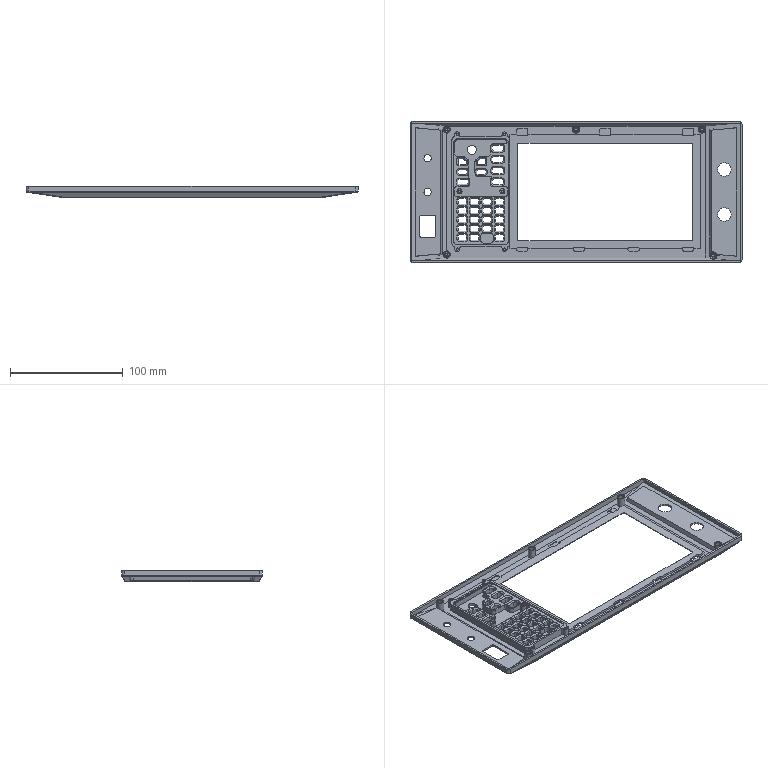NC program | NX | posted with a generic post | part box 295 x 125 x 10 mm
Lines 75 to 1153 of 134431:
(ADAPTIVE_MILLING , TOOL : D10)
N130 T10 M6
N132 G54
N134 G17 G0 G90 X-158.197 Y-0.05 S9500 M3
N136 G43 Z30. H10
N138 Z-7.
N140 G94 G1 Z-10. F1000.
N142 X-156.84 Y-0.58 F3000.
N144 G3 X-155.55 Y-0.05 R1.015
N146 X-154.906 Y3.11 R9.424
N148 X-154.71 Y14.606 R185.073
N150 G1 X-154.708 Y20.006
N152 Y62.706
N154 X-154.706 Y62.906
N156 X-154.702 Y63.006
N158 X-154.696 Y63.105
N160 X-154.687 Y63.205
N162 G2 X-151.776 Y67.539 R6.032
N164 X-146.207 Y69.327 R13.14
N166 X-137.719 Y69.675 R79.253
N168 G1 X-136.319 Y69.682
N170 X-134.219 Y69.687
N172 X-130.719 Y69.69
N174 X-118.819 Y69.691
N176 X-50.119
N178 X-49.119 Y69.695
N180 X-47.519 Y69.697
N182 X-46.119 Y69.696
N184 X-45.419 Y69.698
N186 X-44.319 Y69.697
N188 X-43.319 Y69.699
N190 X-42.519 Y69.698
N192 X-41.619 Y69.7
N194 X-40.719 Y69.699
N196 X-39.819 Y69.7
N198 X-38.819 Y69.699
N200 X-37.719 Y69.701
N202 X-36.719 Y69.699
N204 X-35.719 Y69.7
N206 X-34.219 Y69.698
N208 X-33.319 Y69.7
N210 X-32.319 Y69.699
N212 X-31.419 Y69.7
N214 X-30.319 Y69.698
N216 X-29.519 Y69.7
N218 X-28.619 Y69.699
N220 X-27.619 Y69.7
N222 X-26.719 Y69.699
N224 X-25.719 Y69.7
N226 X-24.819 Y69.699
N228 X-23.819 Y69.7
N230 X-22.719 Y69.698
N232 X-21.719 Y69.699
N234 X-20.219 Y69.698
N236 X-19.219 Y69.7
N238 X-18.219 Y69.699
N240 X-16.719 Y69.701
N242 X-15.719 Y69.699
N244 X-14.619 Y69.701
N246 X-13.619 Y69.699
N248 X-12.619 Y69.7
N250 X-11.219 Y69.698
N252 X-10.219 Y69.7
N254 X-9.219 Y69.698
N256 X-8.219 Y69.699
N258 X-6.719 Y69.698
N260 X-5.619 Y69.7
N262 X-4.519 Y69.698
N264 X-3.519 Y69.7
N266 X-2.519 Y69.699
N268 X-1.019 Y69.701
N270 X-0.119 Y69.699
N272 X0.881 Y69.701
N274 X1.781 Y69.7
N276 X2.881 Y69.701
N278 X3.681 Y69.699
N280 X4.581 Y69.7
N282 X5.581 Y69.698
N284 X6.481 Y69.7
N286 X7.581 Y69.698
N288 X8.581 Y69.699
N290 X10.081 Y69.698
N292 X11.081 Y69.7
N294 X12.081 Y69.699
N296 X13.681 Y69.701
N298 X14.481 Y69.699
N300 X15.581 Y69.701
N302 X16.681 Y69.699
N304 X17.581 Y69.701
N306 X18.581 Y69.699
N308 X19.481 Y69.7
N310 X20.581 Y69.698
N312 X21.381 Y69.7
N314 X22.481 Y69.698
N316 X23.281 Y69.7
N318 X24.381 Y69.698
N320 X25.381 Y69.699
N322 X26.581 Y69.698
N324 X27.081
N326 X27.881 Y69.699
N328 X28.881 Y69.698
N330 X29.781 Y69.699
N332 X30.781 Y69.698
N334 X31.881 Y69.7
N336 X32.881 Y69.698
N338 X33.881 Y69.699
N340 X35.381 Y69.698
N342 X36.381 Y69.7
N344 X37.481 Y69.698
N346 X38.281 Y69.7
N348 X39.381 Y69.698
N350 X40.481 Y69.7
N352 X41.381 Y69.699
N354 X42.281
N356 X43.381 Y69.698
N358 X44.181 Y69.699
N360 X45.081
N362 X46.081 Y69.701
N364 X46.981 Y69.699
N366 X48.081 Y69.701
N368 X49.081 Y69.7
N370 X50.281 Y69.701
N372 X50.781
N374 X51.581 Y69.7
N376 X52.581 Y69.701
N378 X53.481 Y69.699
N380 X54.581 Y69.701
N382 X55.481 Y69.699
N384 X56.581 Y69.7
N386 X57.481 Y69.699
N388 X58.381 Y69.7
N390 X59.481 Y69.698
N392 X60.281 Y69.7
N394 X61.181 Y69.699
N396 X62.081 Y69.7
N398 X63.081 Y69.698
N400 X64.081 Y69.7
N402 X64.981 Y69.699
N404 X65.981 Y69.7
N406 X66.981 Y69.699
N408 X67.881 Y69.7
N410 X68.981 Y69.698
N412 X69.981 Y69.7
N414 X71.081 Y69.698
N416 X72.081 Y69.7
N418 X73.081 Y69.699
N420 X74.481 Y69.701
N422 X75.481 Y69.699
N424 X76.481 Y69.701
N426 X77.481 Y69.7
N428 X78.981 Y69.701
N430 X80.081 Y69.699
N432 X81.181 Y69.701
N434 X82.181 Y69.699
N436 X83.181 Y69.7
N438 X84.681 Y69.698
N440 X85.581 Y69.7
N442 X86.581 Y69.698
N444 X87.481 Y69.699
N446 X88.581 Y69.698
N448 X89.381 Y69.7
N450 X90.281 Y69.699
N452 X91.281 Y69.7
N454 X92.181 Y69.699
N456 X93.081 Y69.7
N458 X94.081 Y69.698
N460 X95.181 Y69.701
N462 X96.281 Y69.698
N464 X97.381 Y69.701
N466 X98.481 Y69.698
N468 X99.581 Y69.701
N470 X100.581 Y69.699
N472 X101.581 Y69.7
N474 X103.181 Y69.698
N476 X103.981 Y69.699
N478 X105.081 Y69.698
N480 X105.881 Y69.699
N482 X106.981 Y69.698
N484 X108.181 Y69.7
N486 X109.181 Y69.698
N488 X110.181 Y69.699
N490 X111.281 Y69.698
N492 X111.781
N494 X112.581 Y69.699
N496 X113.681 Y69.697
N498 X114.681 Y69.699
N500 X115.881 Y69.698
N502 X116.381 Y69.697
N504 X117.181 Y69.699
N506 X118.181 Y69.698
N508 X118.981 Y69.699
N510 X120.081 Y69.698
N512 X120.981 Y69.7
N514 X121.981 Y69.698
N516 X122.981 Y69.7
N518 X124.081 Y69.698
N520 X125.081 Y69.7
N522 X126.081 Y69.699
N524 X127.481 Y69.701
N526 X128.481 Y69.699
N528 X129.481 Y69.701
N530 X130.481 Y69.7
N532 X131.981 Y69.701
N534 X132.981 Y69.699
N536 X134.081 Y69.701
N538 X135.081 Y69.699
N540 X136.081 Y69.7
N542 X137.681 Y69.698
N544 X138.581 Y69.699
N546 X140.181 Y69.697
N548 X141.081 Y69.699
N550 X142.581 Y69.697
N552 X143.481 Y69.7
N554 X144.481 Y69.698
N556 X145.481 Y69.7
N558 X146.481 Y69.698
N560 G2 X149.159 Y69.487 R8.7
N562 X153.113 Y65.746 R6.824
N564 X154.466 Y59.832 R16.868
N566 X154.685 Y49.837 R152.1
N568 G1 X154.689 Y46.937
N570 X154.691 Y39.937
N572 Y-17.563
N574 X154.695 Y-18.563
N576 X154.697 Y-20.163
N578 X154.696 Y-21.563
N580 X154.698 Y-22.263
N582 X154.697 Y-23.363
N584 X154.699 Y-24.363
N586 Y-25.263
N588 X154.7 Y-26.263
N590 X154.699 Y-27.163
N592 X154.7 Y-28.063
N594 X154.699 Y-28.963
N596 X154.7 Y-29.863
N598 X154.699 Y-30.863
N600 X154.7 Y-31.863
N602 X154.698 Y-32.763
N604 X154.7 Y-33.663
N606 X154.698 Y-34.763
N608 X154.699 Y-35.563
N610 X154.698 Y-36.663
N612 X154.699 Y-37.463
N614 X154.698 Y-38.563
N616 X154.699 Y-39.363
N618 X154.698 Y-40.463
N620 X154.7 Y-41.563
N622 X154.698 Y-42.663
N624 X154.7 Y-43.663
N626 X154.699 Y-44.663
N628 X154.701 Y-46.063
N630 X154.698 Y-47.063
N632 X154.701 Y-48.263
N634 X154.699 Y-49.163
N636 X154.701 Y-50.163
N638 X154.7 Y-51.063
N640 X154.701 Y-52.063
N642 Y-52.663
N644 X154.7 Y-53.563
N646 X154.701 Y-54.963
N648 X154.699 Y-55.963
N650 X154.701 Y-57.063
N652 X154.699 Y-57.863
N654 X154.701 Y-58.963
N656 X154.699 Y-59.963
N658 X154.7 Y-61.063
N660 X154.699 Y-61.863
N662 X154.701 Y-62.663
N664 X154.7 Y-62.863
N666 X154.696 Y-62.963
N668 X154.691 Y-63.063
N670 X154.684 Y-63.162
N672 X154.674 Y-63.262
N674 G2 X151.636 Y-67.624 R6.119
N676 X145.844 Y-69.369 R13.739
N678 X136.053 Y-69.682 R100.968
N680 G1 X133.853 Y-69.687
N682 X130.153 Y-69.69
N684 X113.753 Y-69.691
N686 X-26.547
N688 X-27.547 Y-69.695
N690 X-29.147 Y-69.697
N692 X-30.647 Y-69.695
N694 X-31.547 Y-69.698
N696 X-32.447
N698 X-33.547 Y-69.7
N700 X-34.547 Y-69.698
N702 X-35.447 Y-69.7
N704 X-36.547 Y-69.698
N706 X-37.447 Y-69.7
N708 X-38.447 Y-69.698
N710 X-39.547 Y-69.701
N712 X-40.547 Y-69.699
N714 X-41.647 Y-69.7
N716 X-42.447 Y-69.699
N718 X-43.447 Y-69.7
N720 X-44.447 Y-69.699
N722 X-45.447 Y-69.701
N724 X-46.547 Y-69.699
N726 X-47.347 Y-69.7
N728 X-48.447 Y-69.698
N730 X-49.447 Y-69.7
N732 X-50.347 Y-69.698
N734 X-51.247 Y-69.7
N736 X-52.247 Y-69.698
N738 X-53.147 Y-69.7
N740 X-54.047 Y-69.699
N742 X-54.947 Y-69.7
N744 X-55.847 Y-69.699
N746 X-56.647 Y-69.7
N748 X-57.647 Y-69.698
N750 X-58.747 Y-69.701
N752 X-59.747 Y-69.699
N754 X-60.747 Y-69.7
N756 X-62.247 Y-69.698
N758 X-63.147 Y-69.7
N760 X-64.147 Y-69.699
N762 X-65.147 Y-69.7
N764 X-66.047 Y-69.699
N766 X-67.047 Y-69.701
N768 X-68.247 Y-69.698
N770 X-69.147 Y-69.7
N772 X-70.147 Y-69.699
N774 X-71.147 Y-69.7
N776 X-72.147 Y-69.698
N778 X-73.147 Y-69.699
N780 X-74.747 Y-69.698
N782 X-75.447 Y-69.699
N784 X-76.647 Y-69.698
N786 X-77.647 Y-69.7
N788 X-78.747 Y-69.698
N790 X-79.547 Y-69.7
N792 X-80.547 Y-69.699
N794 X-81.447 Y-69.7
N796 X-82.247 Y-69.699
N798 X-83.247 Y-69.7
N800 X-84.347 Y-69.699
N802 X-85.247 Y-69.7
N804 X-86.247 Y-69.699
N806 X-87.147 Y-69.7
N808 X-88.047 Y-69.699
N810 X-89.047 Y-69.701
N812 X-90.047 Y-69.699
N814 X-91.247 Y-69.701
N816 X-92.147 Y-69.699
N818 X-93.147 Y-69.701
N820 X-94.047 Y-69.7
N822 X-95.047 Y-69.701
N824 X-95.647
N826 X-96.547 Y-69.699
N828 X-97.447 Y-69.7
N830 X-98.447 Y-69.699
N832 X-99.547 Y-69.701
N834 X-100.447 Y-69.699
N836 X-101.447 Y-69.701
N838 X-102.447 Y-69.699
N840 X-103.347 Y-69.701
N842 X-104.247 Y-69.699
N844 X-105.246 Y-69.701
N846 X-106.246 Y-69.698
N848 X-107.246 Y-69.7
N850 X-108.846 Y-69.698
N852 X-109.646 Y-69.699
N854 X-110.746 Y-69.698
N856 X-111.946 Y-69.7
N858 X-112.946 Y-69.698
N860 X-113.946 Y-69.699
N862 X-115.446 Y-69.698
N864 X-116.346 Y-69.7
N866 X-117.346 Y-69.698
N868 X-118.246 Y-69.7
N870 X-119.146 Y-69.699
N872 X-120.146 Y-69.7
N874 X-121.146 Y-69.699
N876 X-122.146 Y-69.701
N878 X-123.246 Y-69.699
N880 X-124.046 Y-69.7
N882 X-125.146 Y-69.698
N884 X-126.146 Y-69.7
N886 X-127.046 Y-69.698
N888 X-127.946 Y-69.7
N890 X-129.046 Y-69.698
N892 X-129.846 Y-69.7
N894 X-130.946 Y-69.698
N896 X-131.746 Y-69.699
N898 X-132.846 Y-69.698
N900 X-133.946 Y-69.7
N902 X-134.946 Y-69.698
N904 X-136.046 Y-69.7
N906 X-136.846 Y-69.699
N908 X-137.946 Y-69.701
N910 X-138.746 Y-69.699
N912 X-139.846 Y-69.701
N914 X-140.646 Y-69.699
N916 X-141.746 Y-69.701
N918 X-142.546 Y-69.7
N920 X-143.646 Y-69.701
N922 X-144.846 Y-69.699
N924 G2 X-148.543 Y-69.636 R33.101
N926 X-152.72 Y-66.482 R6.279
N928 X-154.388 Y-60.664 R14.238
N930 X-154.681 Y-51.272 R104.043
N932 G1 X-154.686 Y-49.272
N934 X-154.69 Y-45.872
N936 X-154.691 Y-35.572
N938 Y-3.372
N940 X-154.685 Y-3.072
N942 X-154.679 Y-2.873
N944 G3 X-154.122 Y3.603 R975.318
N946 X-153.919 Y17.399 R287.72
N948 G1 X-153.917 Y22.999
N950 Y59.999
N952 X-153.914 Y60.199
N954 X-153.907 Y60.399
N956 X-153.894 Y60.599
N958 G2 X-150.004 Y66.557 R7.684
N960 X-143.743 Y68.482 R15.693
N962 X-134.055 Y68.866 R91.543
N964 G1 X-132.455 Y68.873
N966 X-130.155 Y68.878
N968 X-126.455 Y68.881
N970 X-114.555 Y68.882
N972 X-52.855 Y68.883
N974 X-51.655 Y68.889
N976 X-50.255
N978 X-49.355 Y68.892
N980 X-47.855 Y68.893
N982 X-46.955
N984 X-45.955 Y68.896
N986 X-44.955 Y68.895
N988 X-44.155 Y68.897
N990 X-43.055
N992 X-42.155 Y68.899
N994 X-41.255 Y68.898
N996 X-40.155 Y68.9
N998 X-39.255 Y68.899
N1000 X-38.055 Y68.901
N1002 X-36.955 Y68.898
N1004 X-35.855 Y68.9
N1006 X-34.755 Y68.898
N1008 X-33.755 Y68.9
N1010 X-32.855 Y68.899
N1012 X-31.955 Y68.9
N1014 X-30.855 Y68.898
N1016 X-30.055 Y68.9
N1018 X-28.955 Y68.898
N1020 X-27.955 Y68.9
N1022 X-27.155 Y68.899
N1024 X-26.155 Y68.9
N1026 X-25.155 Y68.899
N1028 X-24.155 Y68.9
N1030 X-23.055 Y68.898
N1032 X-21.855 Y68.9
N1034 X-20.855 Y68.899
N1036 X-19.555 Y68.902
N1038 X-18.455 Y68.899
N1040 X-17.255 Y68.901
N1042 X-16.355 Y68.9
N1044 X-14.955 Y68.902
N1046 X-14.055 Y68.899
N1048 X-12.955 Y68.901
N1050 X-11.855 Y68.899
N1052 X-10.855 Y68.9
N1054 X-9.955 Y68.899
N1056 X-8.355 Y68.902
N1058 X-7.155 Y68.899
N1060 X-6.055 Y68.901
N1062 X-5.156 Y68.9
N1064 X-3.756 Y68.902
N1066 X-2.656 Y68.9
N1068 X-1.856 Y68.901
N1070 X-0.856 Y68.9
N1072 X0.144 Y68.901
N1074 X1.044 Y68.9
N1076 X2.044 Y68.901
N1078 X2.944 Y68.9
N1080 X4.044 Y68.901
N1082 X4.944 Y68.899
N1084 X6.144 Y68.901
N1086 X7.244 Y68.898
N1088 X8.544 Y68.9
N1090 X9.444 Y68.898
N1092 X10.644 Y68.901
N1094 X11.744 Y68.898
N1096 X12.944 Y68.901
N1098 X13.844 Y68.9
N1100 X15.044 Y68.901
N1102 X16.144 Y68.899
N1104 X17.044 Y68.9
N1106 X18.044 Y68.899
N1108 X19.044 Y68.9
N1110 X19.944 Y68.899
N1112 X21.144 Y68.9
N1114 X21.944 Y68.899
N1116 X23.244 Y68.9
N1118 X24.244 Y68.898
N1120 X25.344 Y68.9
N1122 X26.444 Y68.898
N1124 X27.444 Y68.899
N1126 X28.244 Y68.898
N1128 X29.344 Y68.9
N1130 X30.344 Y68.898
N1132 X31.244 Y68.899
N1134 X32.544 Y68.897
N1136 X33.644 Y68.899
N1138 X34.844 Y68.898
N1140 X35.744 Y68.899
N1142 X37.144 Y68.897
N1144 X38.044 Y68.899
N1146 X38.944 Y68.898
N1148 X39.944 Y68.9
N1150 X40.944 Y68.898
N1152 X41.944 Y68.9
N1154 X42.844 Y68.898
N1156 X43.844 Y68.9
N1158 X44.944 Y68.899
N1160 X45.844 Y68.901
N1162 X46.944 Y68.899
N1164 X47.944 Y68.901
N1166 X49.044 Y68.899
N1168 X49.944 Y68.901
N1170 X51.044 Y68.899
N1172 X52.044 Y68.901
N1174 X52.944 Y68.899
N1176 X54.044 Y68.9
N1178 X54.944 Y68.899
N1180 X56.044 Y68.901
N1182 X57.144 Y68.898
N1184 X58.144 Y68.9
N1186 X59.044 Y68.899
N1188 X59.944 Y68.9
N1190 X60.944 Y68.898
N1192 X61.844 Y68.9
N1194 X62.744 Y68.899
N1196 X63.644 Y68.9
N1198 X64.644 Y68.899
N1200 X65.544 Y68.9
N1202 X66.644 Y68.898
N1204 X67.644 Y68.9
N1206 X68.644 Y68.898
N1208 X69.644 Y68.9
N1210 X70.544 Y68.899
N1212 X71.744 Y68.901
N1214 X72.844 Y68.899
N1216 X73.944 Y68.901
N1218 X74.944 Y68.9
N1220 X76.044 Y68.901
N1222 X77.344 Y68.898
N1224 X78.444 Y68.901
N1226 X79.644 Y68.899
N1228 X80.644 Y68.9
N1230 X81.744 Y68.898
N1232 X82.944 Y68.9
N1234 X83.944 Y68.898
N1236 X84.844 Y68.9
N1238 X85.744 Y68.899
N1240 X86.944 Y68.901
N1242 X87.844 Y68.899
N1244 X88.944 Y68.9
N1246 X90.144 Y68.899
N1248 X90.944 Y68.9
N1250 X91.844 Y68.899
N1252 X92.844 Y68.9
N1254 X93.844 Y68.899
N1256 X94.944 Y68.9
N1258 X95.944 Y68.899
N1260 X97.044 Y68.9
N1262 X98.144 Y68.899
N1264 X99.244 Y68.9
N1266 X100.344 Y68.898
N1268 X101.444 Y68.9
N1270 X102.544 Y68.898
N1272 X103.344 Y68.899
N1274 X104.444 Y68.897
N1276 X105.544 Y68.899
N1278 X106.744 Y68.898
N1280 X107.844 Y68.9
N1282 X108.944 Y68.897
N1284 X110.044 Y68.9
N1286 X111.144 Y68.897
N1288 X112.244 Y68.899
N1290 X113.344 Y68.897
N1292 X114.544 Y68.9
N1294 X115.644 Y68.898
N1296 X116.644 Y68.9
N1298 X117.544 Y68.898
N1300 X118.644 Y68.9
N1302 X119.644 Y68.898
N1304 X120.644 Y68.9
N1306 X121.744 Y68.898
N1308 X122.644 Y68.9
N1310 X123.644 Y68.898
N1312 X124.844 Y68.901
N1314 X125.944 Y68.899
N1316 X127.044 Y68.901
N1318 X128.144 Y68.899
N1320 X129.244 Y68.902
N1322 X130.444 Y68.899
N1324 X131.544 Y68.901
N1326 X132.644 Y68.899
N1328 X133.544 Y68.9
N1330 X134.944 Y68.898
N1332 X135.944 Y68.899
N1334 X137.144 Y68.897
N1336 X138.144 Y68.899
N1338 X139.744 Y68.895
N1340 X140.944 Y68.898
N1342 X141.744 Y68.897
N1344 X142.844 Y68.899
N1346 X143.944 Y68.898
N1348 X144.844 Y68.899
N1350 X145.144 Y68.898
N1352 X145.244 Y68.896
N1354 X145.344 Y68.893
N1356 X145.444 Y68.888
N1358 X145.544 Y68.883
N1360 X145.644 Y68.875
N1362 G2 X151.529 Y65.037 R7.676
N1364 X153.487 Y58.684 R15.62
N1366 X153.866 Y49.096 R91.104
N1368 G1 X153.873 Y47.296
N1370 X153.878 Y45.096
N1372 X153.881 Y41.296
N1374 X153.882 Y27.496
N1376 X153.883 Y-14.904
N1378 X153.887 Y-16.004
N1380 X153.89 Y-17.504
N1382 Y-18.804
N1384 X153.893 Y-19.704
N1386 Y-20.404
N1388 Y-21.004
N1390 X153.896 Y-21.904
N1392 Y-23.004
N1394 X153.899 Y-24.104
N1396 X153.897 Y-25.004
N1398 X153.9 Y-26.104
N1400 X153.898 Y-27.004
N1402 X153.899 Y-27.904
N1404 X153.898 Y-29.004
N1406 X153.899 Y-29.804
N1408 X153.898 Y-30.904
N1410 X153.899 Y-31.704
N1412 X153.898 Y-32.804
N1414 X153.899 Y-33.704
N1416 X153.898 Y-34.804
N1418 X153.899 Y-35.604
N1420 X153.898 Y-36.404
N1422 X153.899 Y-37.304
N1424 X153.898 Y-38.304
N1426 X153.899 Y-39.304
N1428 X153.898 Y-40.304
N1430 X153.9 Y-41.404
N1432 X153.899 Y-42.304
N1434 X153.901 Y-43.404
N1436 X153.899 Y-44.504
N1438 X153.9 Y-45.504
N1440 X153.898 Y-46.604
N1442 X153.901 Y-47.704
N1444 X153.899 Y-48.804
N1446 X153.901 Y-49.904
N1448 X153.9 Y-51.004
N1450 X153.901 Y-51.904
N1452 X153.898 Y-53.304
N1454 X153.901 Y-54.504
N1456 X153.899 Y-55.504
N1458 X153.901 Y-56.504
N1460 X153.899 Y-57.604
N1462 X153.9 Y-58.604
N1464 X153.898 Y-59.704
N1466 X153.899 Y-60.004
N1468 X153.896 Y-60.204
N1470 X153.889 Y-60.404
N1472 X153.877 Y-60.603
N1474 G2 X149.986 Y-66.559 R7.67
N1476 X143.724 Y-68.482 R15.599
N1478 X133.837 Y-68.867 R92.124
N1480 G1 X132.137 Y-68.874
N1482 X129.737 Y-68.879
N1484 X125.637 Y-68.881
N1486 X106.937 Y-68.882
N1488 X-23.763 Y-68.883
N1490 X-24.863 Y-68.888
N1492 X-26.263 Y-68.889
N1494 X-27.163 Y-68.892
N1496 X-28.663 Y-68.893
N1498 X-29.563
N1500 X-30.663 Y-68.896
N1502 X-31.863 Y-68.895
N1504 X-32.863 Y-68.898
N1506 X-33.963 Y-68.896
N1508 X-34.963 Y-68.899
N1510 X-36.063 Y-68.897
N1512 X-37.063 Y-68.9
N1514 X-38.163 Y-68.898
N1516 X-39.163 Y-68.9
N1518 X-40.063 Y-68.899
N1520 X-41.063 Y-68.9
N1522 X-42.063 Y-68.899
N1524 X-43.063 Y-68.9
N1526 X-44.163 Y-68.898
N1528 X-45.163 Y-68.9
N1530 X-46.163 Y-68.898
N1532 X-47.163 Y-68.9
N1534 X-48.063 Y-68.899
N1536 X-49.063 Y-68.9
N1538 X-49.963 Y-68.899
N1540 X-50.963 Y-68.9
N1542 X-51.863 Y-68.899
N1544 X-52.863 Y-68.9
N1546 X-53.763 Y-68.898
N1548 X-54.663 Y-68.9
N1550 X-55.663 Y-68.899
N1552 X-56.563 Y-68.9
N1554 X-57.563 Y-68.899
N1556 X-58.463 Y-68.9
N1558 X-59.663 Y-68.898
N1560 X-60.763 Y-68.9
N1562 X-61.863 Y-68.898
N1564 X-62.763 Y-68.899
N1566 X-64.063 Y-68.898
N1568 X-64.963 Y-68.9
N1570 X-66.263 Y-68.898
N1572 X-67.163 Y-68.9
N1574 X-68.063 Y-68.898
N1576 X-68.963 Y-68.9
N1578 X-69.863 Y-68.899
N1580 X-70.863 Y-68.9
N1582 X-72.063 Y-68.897
N1584 X-73.063 Y-68.899
N1586 X-74.163 Y-68.897
N1588 X-75.063 Y-68.899
N1590 X-76.163 Y-68.898
N1592 X-77.063 Y-68.899
N1594 X-78.063 Y-68.898
N1596 X-78.963 Y-68.899
N1598 X-79.963 Y-68.898
N1600 X-80.863 Y-68.9
N1602 X-81.963 Y-68.898
N1604 X-82.963 Y-68.9
N1606 X-83.863 Y-68.899
N1608 X-84.963 Y-68.9
N1610 X-85.963 Y-68.899
N1612 X-86.863 Y-68.9
N1614 X-88.063 Y-68.898
N1616 X-88.963 Y-68.9
N1618 X-89.863 Y-68.899
N1620 X-90.863 Y-68.901
N1622 X-91.763 Y-68.9
N1624 X-92.963 Y-68.902
N1626 X-93.963 Y-68.9
N1628 X-94.963 Y-68.901
N1630 X-95.863 Y-68.9
N1632 X-97.063 Y-68.902
N1634 X-98.063 Y-68.9
N1636 X-98.963 Y-68.901
N1638 X-100.063 Y-68.899
N1640 X-100.963 Y-68.9
N1642 X-102.063 Y-68.899
N1644 X-103.063 Y-68.9
N1646 X-104.163 Y-68.898
N1648 X-105.063 Y-68.9
N1650 X-106.363 Y-68.898
N1652 X-107.363 Y-68.9
N1654 X-108.463 Y-68.898
N1656 X-109.563 Y-68.9
N1658 X-110.563 Y-68.898
N1660 X-111.663 Y-68.9
N1662 X-112.763 Y-68.898
N1664 X-113.863 Y-68.9
N1666 X-114.963 Y-68.898
N1668 X-115.763 Y-68.899
N1670 X-116.863 Y-68.898
N1672 X-117.763 Y-68.9
N1674 X-118.763 Y-68.898
N1676 X-119.663 Y-68.9
N1678 X-120.763 Y-68.899
N1680 X-121.663 Y-68.9
N1682 X-122.763 Y-68.898
N1684 X-123.763 Y-68.9
N1686 X-124.663 Y-68.899
N1688 X-125.763 Y-68.9
N1690 X-126.763 Y-68.899
N1692 X-127.563 Y-68.9
N1694 X-128.563 Y-68.898
N1696 X-129.563 Y-68.9
N1698 X-130.463 Y-68.898
N1700 X-131.563 Y-68.9
N1702 X-132.663 Y-68.898
N1704 X-133.563 Y-68.9
N1706 X-134.663 Y-68.898
N1708 X-135.663 Y-68.9
N1710 X-136.463 Y-68.899
N1712 X-137.463 Y-68.901
N1714 X-138.363 Y-68.899
N1716 X-139.463 Y-68.901
N1718 X-140.263 Y-68.9
N1720 G2 X-145.861 Y-68.855 R109.006
N1722 X-151.692 Y-64.765 R7.777
N1724 X-153.499 Y-58.567 R16.186
N1726 X-153.866 Y-49.079 R92.965
N1728 G1 X-153.873 Y-47.479
N1730 X-153.877 Y-45.379
N1732 X-153.881 Y-41.779
N1734 X-153.882 Y-31.879
N1736 Y-5.479
N1738 X-153.88 Y-5.279
N1740 G2 X-153.385 Y2.905 R186.247
N1742 G3 X-153.131 Y17.201 R283.875
N1744 G1 X-153.127 Y20.801
N1746 X-153.125 Y29.001
N1748 Y57.401
N1750 X-153.123 Y57.701
N1752 X-153.12 Y57.901
N1754 X-153.115 Y58.101
N1756 G2 X-152.511 Y61.232 R9.849
N1758 G1 X-152.465 Y61.644
N1760 X-152.439 Y61.758
N1762 G2 X-150.939 Y64.811 R8.761
N1764 X-148.264 Y66.912 R8.761
N1766 G1 X-146.758 Y67.439
N1768 X-146.644 Y67.465
N1770 G2 X-135.28 Y68.033 R103.719
N1772 G1 X-134.08 Y68.045
N1774 X-132.78 Y68.054
N1776 X-131.08 Y68.062
N1778 X-128.78 Y68.068
N1780 X-125.38 Y68.072
N1782 X-118.38 Y68.073
N1784 X-55.58 Y68.074
N1786 X-54.68 Y68.078
N1788 X-53.28 Y68.08
N1790 X-52.78 Y68.081
N1792 X-51.78 Y68.085
N1794 X-50.38 Y68.087
N1796 X-49.38
N1798 X-48.58 Y68.09
N1800 X-47.88 Y68.091
N1802 X-47.28
N1804 X-46.38 Y68.094
N1806 X-45.28
N1808 X-44.38 Y68.096
N1810 X-43.28 Y68.095
N1812 X-42.38 Y68.098
N1814 X-41.38 Y68.097
N1816 X-40.48 Y68.099
N1818 X-39.68 Y68.098
N1820 X-39.08
N1822 X-38.18 Y68.1
N1824 X-37.18 Y68.099
N1826 X-35.98 Y68.101
N1828 X-34.98 Y68.099
N1830 X-33.98 Y68.1
N1832 X-32.98 Y68.098
N1834 X-31.98 Y68.1
N1836 X-31.08 Y68.098
N1838 X-30.18 Y68.1
N1840 X-29.18 Y68.098
N1842 X-28.28 Y68.1
N1844 X-27.18 Y68.098
N1846 X-26.18 Y68.1
N1848 X-25.18 Y68.098
N1850 X-24.18 Y68.099
N1852 X-23.08 Y68.098
N1854 X-21.88 Y68.101
N1856 X-20.78 Y68.099
N1858 X-19.78 Y68.1
N1860 X-18.78 Y68.099
N1862 X-17.58 Y68.102
N1864 X-16.38 Y68.099
N1866 X-15.48 Y68.101
N1868 X-14.28 Y68.099
N1870 X-13.28 Y68.1
N1872 X-12.38 Y68.099
N1874 X-11.78 Y68.1
N1876 X-11.18 Y68.102
N1878 X-10.68 Y68.101
N1880 X-9.78 Y68.099
N1882 X-8.68 Y68.101
N1884 X-7.68 Y68.099
N1886 X-6.38 Y68.102
N1888 X-5.18 Y68.099
N1890 X-4.08 Y68.101
N1892 X-3.28 Y68.1
N1894 X-2.18 Y68.101
N1896 X-1.28 Y68.1
N1898 X-0.28 Y68.101
N1900 X0.92 Y68.099
N1902 X1.82 Y68.1
N1904 X3.02 Y68.099
N1906 X3.92 Y68.1
N1908 X5.12 Y68.098
N1910 X6.12 Y68.1
N1912 X7.22 Y68.099
N1914 X8.42 Y68.101
N1916 X9.52 Y68.099
N1918 X10.62 Y68.101
N1920 X11.42 Y68.1
N1922 X12.52 Y68.101
N1924 X13.62 Y68.099
N1926 X14.72 Y68.101
N1928 X15.72 Y68.099
N1930 X16.72 Y68.1
N1932 X17.62 Y68.099
N1934 X18.72 Y68.1
N1936 X19.72 Y68.099
N1938 X20.82 Y68.1
N1940 X21.92 Y68.099
N1942 X22.92 Y68.1
N1944 X24.02 Y68.098
N1946 X25.02 Y68.099
N1948 X26.12 Y68.098
N1950 X27.12 Y68.099
N1952 X28.02 Y68.098
N1954 X29.12 Y68.1
N1956 X30.12 Y68.098
N1958 X30.82 Y68.099
N1960 X31.32 Y68.1
N1962 X32.32 Y68.098
N1964 X33.32 Y68.099
N1966 X34.62 Y68.097
N1968 X35.52 Y68.099
N1970 X36.62 Y68.097
N1972 X37.62 Y68.099
N1974 X38.72 Y68.098
N1976 X39.82 Y68.1
N1978 X40.72 Y68.099
N1980 X42.12 Y68.1
N1982 X42.92 Y68.099
N1984 X43.92 Y68.101
N1986 X44.92 Y68.099
N1988 X45.82 Y68.101
N1990 X46.82 Y68.099
N1992 X47.72 Y68.1
N1994 X48.72 Y68.099
N1996 X49.82 Y68.101
N1998 X50.72 Y68.099
N2000 X51.82 Y68.101
N2002 X52.92 Y68.099
N2004 X53.82 Y68.1
N2006 X55.22 Y68.099
N2008 X56.12 Y68.1
N2010 X57.42 Y68.098
N2012 X58.22 Y68.099
N2014 X59.22 Y68.098
N2016 X60.02 Y68.096
N2018 X61.02 Y68.099
N2020 X62.12 Y68.098
N2022 X63.02 Y68.099
N2024 X64.22 Y68.097
N2026 X65.22 Y68.099
N2028 X66.42 Y68.097
N2030 X67.42 Y68.099
N2032 X68.52 Y68.098
N2034 X69.32 Y68.099
N2036 X70.02
N2038 X70.52 Y68.098
N2040 X71.62 Y68.1
N2042 X72.62 Y68.099
N2044 X73.62 Y68.101
N2046 X74.22 Y68.1
N2048 X74.82 Y68.099
N2050 X75.92 Y68.1
N2052 X77.12 Y68.098
N2054 X78.12 Y68.1
N2056 X79.22 Y68.099
N2058 X80.42 Y68.101
N2060 X81.52 Y68.098
N2062 X82.52 Y68.1
N2064 X83.52 Y68.099
N2066 X84.52 Y68.1
N2068 X85.62 Y68.099
N2070 X86.72 Y68.101
N2072 X87.72 Y68.099
N2074 X88.72 Y68.1
N2076 X89.82 Y68.098
N2078 X90.72 Y68.1
N2080 X91.82 Y68.098
N2082 X92.72 Y68.1
N2084 X93.82 Y68.098
N2086 X94.82 Y68.1
N2088 X95.92 Y68.098
N2090 X96.92 Y68.1
N2092 X98.12 Y68.098
N2094 X99.12 Y68.1
N2096 X100.22 Y68.098
N2098 X101.12 Y68.099
N2100 X102.22 Y68.097
N2102 X103.12 Y68.098
N2104 X104.32 Y68.097
N2106 X105.32 Y68.099
N2108 X106.42 Y68.097
N2110 X107.72 Y68.1
N2112 X108.62 Y68.098
N2114 X109.72 Y68.099
N2116 X110.82 Y68.097
N2118 X111.92 Y68.099
N2120 X113.12 Y68.097
N2122 X114.22 Y68.099
N2124 X115.32 Y68.098
N2126 X116.22 Y68.099
N2128 X117.32 Y68.098
N2130 X118.32 Y68.099
N2132 X119.42 Y68.098
N2134 X120.32 Y68.099
N2136 X121.42 Y68.098
N2138 X122.42 Y68.1
N2140 X123.22 Y68.099
N2142 X123.82 Y68.098
N2144 X124.62 Y68.1
N2146 X125.72 Y68.099
N2148 X126.82 Y68.101
N2150 X128.02 Y68.099
N2152 X129.02 Y68.1
N2154 G2 X143.619 Y68.065 R855.271
N2156 X146.153 Y67.52 R10.172
N2158 G1 X146.644 Y67.465
N2160 X146.758 Y67.439
N2162 G2 X149.811 Y65.939 R8.761
N2164 X151.912 Y63.264 R8.761
N2166 G1 X152.439 Y61.758
N2168 X152.465 Y61.644
N2170 G2 X153.032 Y50.38 R102.986
N2172 G1 X153.044 Y49.18
N2174 X153.054 Y47.78
N2176 X153.062 Y46.08
N2178 X153.068 Y43.78
N2180 X153.072 Y40.28
N2182 X153.073 Y32.88
N2184 X153.074 Y-12.22
N2186 X153.078 Y-13.12
N2188 X153.081 Y-14.32
N2190 X153.084 Y-15.12
N2192 Y-16.32
N2194 X153.088 Y-17.32
N2196 Y-18.42
N2198 X153.092 Y-19.42
N2200 Y-20.72
N2202 X153.095 Y-21.72
N2204 X153.096 Y-22.92
N2206 X153.098 Y-24.12
N2208 X153.097 Y-25.02
N2210 X153.098 Y-25.92
N2212 X153.097 Y-27.02
N2214 X153.099 Y-27.82
N2216 X153.098 Y-28.82
N2218 X153.099 Y-29.72
N2220 X153.097 Y-30.82
N2222 X153.099 Y-31.72
N2224 X153.098 Y-32.62
N2226 X153.099 Y-33.52
N2228 X153.098 Y-34.42
N2230 X153.099 Y-35.42
N2232 X153.098 Y-36.22
N2234 X153.099 Y-37.22
N2236 X153.098 Y-38.12
N2238 X153.1 Y-39.12
N2240 X153.098 Y-40.12
N2242 X153.1 Y-41.12
N2244 X153.098 Y-42.22
N2246 X153.1 Y-43.22
N2248 X153.098 Y-44.22
N2250 X153.1 Y-45.32
N2252 X153.098 Y-46.32
N2254 X153.101 Y-47.62
N2256 X153.099 Y-48.62
N2258 X153.1 Y-49.62
N2260 X153.099 Y-50.82
N2262 X153.101 Y-51.92
N2264 X153.099 Y-52.92
N2266 G2 X153.026 Y-59.017 R84.327
N2268 X152.52 Y-61.153 R11.024
N2270 G1 X152.465 Y-61.644
N2272 X152.439 Y-61.758
N2274 G2 X150.939 Y-64.811 R8.761
N2276 X148.264 Y-66.912 R8.761
N2278 G1 X146.758 Y-67.439
N2280 X146.644 Y-67.465